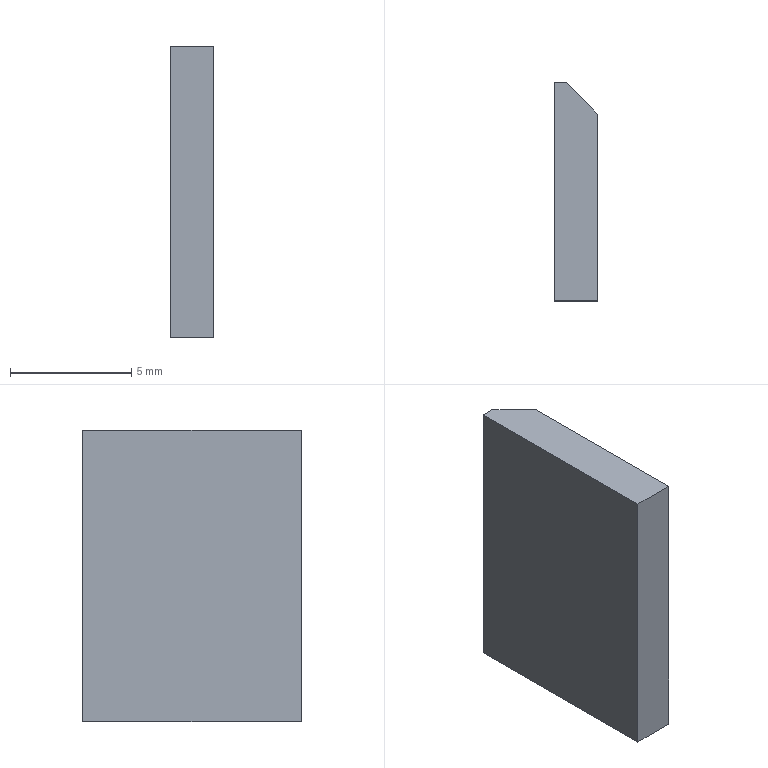Part | SolidWorks | features Extrusion 1 | 1 solid | 7 faces | box 1.8 x 9 x 12 mm | volume 184.26 mm3 | plane 7
STEP:
#1=CARTESIAN_POINT('',(0.5,9.,0.));
#2=VERTEX_POINT('',#1);
#3=CARTESIAN_POINT('',(0.,9.,0.));
#4=VERTEX_POINT('',#3);
#5=CARTESIAN_POINT('',(0.5,9.,0.));
#6=DIRECTION('',(-1.,0.,0.));
#7=VECTOR('',#6,1000.);
#8=LINE('',#5,#7);
#9=EDGE_CURVE('',#2,#4,#8,.T.);
#10=ORIENTED_EDGE('',*,*,#9,.T.);
#11=CARTESIAN_POINT('',(0.,9.,12.));
#12=VERTEX_POINT('',#11);
#13=CARTESIAN_POINT('',(0.,9.,12.));
#14=DIRECTION('',(0.,0.,-1.));
#15=VECTOR('',#14,1000.);
#16=LINE('',#13,#15);
#17=EDGE_CURVE('',#12,#4,#16,.T.);
#18=ORIENTED_EDGE('',*,*,#17,.F.);
#19=CARTESIAN_POINT('',(0.5,9.,12.));
#20=VERTEX_POINT('',#19);
#21=CARTESIAN_POINT('',(0.5,9.,12.));
#22=DIRECTION('',(-1.,0.,0.));
#23=VECTOR('',#22,1000.);
#24=LINE('',#21,#23);
#25=EDGE_CURVE('',#20,#12,#24,.T.);
#26=ORIENTED_EDGE('',*,*,#25,.F.);
#27=CARTESIAN_POINT('',(0.5,9.,12.));
#28=DIRECTION('',(0.,0.,-1.));
#29=VECTOR('',#28,1000.);
#30=LINE('',#27,#29);
#31=EDGE_CURVE('',#20,#2,#30,.T.);
#32=ORIENTED_EDGE('',*,*,#31,.T.);
#33=EDGE_LOOP('',(#10,#18,#26,#32));
#34=FACE_OUTER_BOUND('',#33,.T.);
#35=CARTESIAN_POINT('',(0.5,9.,12.));
#36=DIRECTION('',(0.,-1.,0.));
#37=DIRECTION('',(0.,0.,-1.));
#38=AXIS2_PLACEMENT_3D('',#35,#36,#37);
#39=PLANE('',#38);
#40=ADVANCED_FACE('',(#34),#39,.F.);
#41=CARTESIAN_POINT('',(0.,0.,0.));
#42=VERTEX_POINT('',#41);
#43=CARTESIAN_POINT('',(0.,9.,0.));
#44=DIRECTION('',(0.,-1.,0.));
#45=VECTOR('',#44,1000.);
#46=LINE('',#43,#45);
#47=EDGE_CURVE('',#4,#42,#46,.T.);
#48=ORIENTED_EDGE('',*,*,#47,.T.);
#49=CARTESIAN_POINT('',(0.,0.,12.));
#50=VERTEX_POINT('',#49);
#51=CARTESIAN_POINT('',(0.,0.,12.));
#52=DIRECTION('',(0.,0.,-1.));
#53=VECTOR('',#52,1000.);
#54=LINE('',#51,#53);
#55=EDGE_CURVE('',#50,#42,#54,.T.);
#56=ORIENTED_EDGE('',*,*,#55,.F.);
#57=CARTESIAN_POINT('',(0.,9.,12.));
#58=DIRECTION('',(0.,-1.,0.));
#59=VECTOR('',#58,1000.);
#60=LINE('',#57,#59);
#61=EDGE_CURVE('',#12,#50,#60,.T.);
#62=ORIENTED_EDGE('',*,*,#61,.F.);
#63=ORIENTED_EDGE('',*,*,#17,.T.);
#64=EDGE_LOOP('',(#48,#56,#62,#63));
#65=FACE_OUTER_BOUND('',#64,.T.);
#66=CARTESIAN_POINT('',(0.,9.,12.));
#67=DIRECTION('',(1.,0.,0.));
#68=DIRECTION('',(0.,0.,-1.));
#69=AXIS2_PLACEMENT_3D('',#66,#67,#68);
#70=PLANE('',#69);
#71=ADVANCED_FACE('',(#65),#70,.F.);
#72=CARTESIAN_POINT('',(1.8,0.,0.));
#73=VERTEX_POINT('',#72);
#74=CARTESIAN_POINT('',(0.,0.,0.));
#75=DIRECTION('',(1.,0.,0.));
#76=VECTOR('',#75,1000.);
#77=LINE('',#74,#76);
#78=EDGE_CURVE('',#42,#73,#77,.T.);
#79=ORIENTED_EDGE('',*,*,#78,.T.);
#80=CARTESIAN_POINT('',(1.8,0.,12.));
#81=VERTEX_POINT('',#80);
#82=CARTESIAN_POINT('',(1.8,0.,12.));
#83=DIRECTION('',(0.,0.,-1.));
#84=VECTOR('',#83,1000.);
#85=LINE('',#82,#84);
#86=EDGE_CURVE('',#81,#73,#85,.T.);
#87=ORIENTED_EDGE('',*,*,#86,.F.);
#88=CARTESIAN_POINT('',(0.,0.,12.));
#89=DIRECTION('',(1.,0.,0.));
#90=VECTOR('',#89,1000.);
#91=LINE('',#88,#90);
#92=EDGE_CURVE('',#50,#81,#91,.T.);
#93=ORIENTED_EDGE('',*,*,#92,.F.);
#94=ORIENTED_EDGE('',*,*,#55,.T.);
#95=EDGE_LOOP('',(#79,#87,#93,#94));
#96=FACE_OUTER_BOUND('',#95,.T.);
#97=CARTESIAN_POINT('',(0.,0.,12.));
#98=DIRECTION('',(0.,1.,0.));
#99=DIRECTION('',(0.,0.,1.));
#100=AXIS2_PLACEMENT_3D('',#97,#98,#99);
#101=PLANE('',#100);
#102=ADVANCED_FACE('',(#96),#101,.F.);
#103=CARTESIAN_POINT('',(1.8,7.7,0.));
#104=VERTEX_POINT('',#103);
#105=CARTESIAN_POINT('',(1.8,0.,0.));
#106=DIRECTION('',(0.,1.,0.));
#107=VECTOR('',#106,1000.);
#108=LINE('',#105,#107);
#109=EDGE_CURVE('',#73,#104,#108,.T.);
#110=ORIENTED_EDGE('',*,*,#109,.T.);
#111=CARTESIAN_POINT('',(1.8,7.7,12.));
#112=VERTEX_POINT('',#111);
#113=CARTESIAN_POINT('',(1.8,7.7,12.));
#114=DIRECTION('',(0.,0.,-1.));
#115=VECTOR('',#114,1000.);
#116=LINE('',#113,#115);
#117=EDGE_CURVE('',#112,#104,#116,.T.);
#118=ORIENTED_EDGE('',*,*,#117,.F.);
#119=CARTESIAN_POINT('',(1.8,0.,12.));
#120=DIRECTION('',(0.,1.,0.));
#121=VECTOR('',#120,1000.);
#122=LINE('',#119,#121);
#123=EDGE_CURVE('',#81,#112,#122,.T.);
#124=ORIENTED_EDGE('',*,*,#123,.F.);
#125=ORIENTED_EDGE('',*,*,#86,.T.);
#126=EDGE_LOOP('',(#110,#118,#124,#125));
#127=FACE_OUTER_BOUND('',#126,.T.);
#128=CARTESIAN_POINT('',(1.8,0.,12.));
#129=DIRECTION('',(-1.,0.,0.));
#130=DIRECTION('',(0.,-1.,0.));
#131=AXIS2_PLACEMENT_3D('',#128,#129,#130);
#132=PLANE('',#131);
#133=ADVANCED_FACE('',(#127),#132,.F.);
#134=CARTESIAN_POINT('',(1.8,7.7,0.));
#135=DIRECTION('',(-0.7071,0.7071,0.));
#136=VECTOR('',#135,1000.);
#137=LINE('',#134,#136);
#138=EDGE_CURVE('',#104,#2,#137,.T.);
#139=ORIENTED_EDGE('',*,*,#138,.T.);
#140=ORIENTED_EDGE('',*,*,#31,.F.);
#141=CARTESIAN_POINT('',(1.8,7.7,12.));
#142=DIRECTION('',(-0.7071,0.7071,0.));
#143=VECTOR('',#142,1000.);
#144=LINE('',#141,#143);
#145=EDGE_CURVE('',#112,#20,#144,.T.);
#146=ORIENTED_EDGE('',*,*,#145,.F.);
#147=ORIENTED_EDGE('',*,*,#117,.T.);
#148=EDGE_LOOP('',(#139,#140,#146,#147));
#149=FACE_OUTER_BOUND('',#148,.T.);
#150=CARTESIAN_POINT('',(1.8,7.7,12.));
#151=DIRECTION('',(-0.7071,-0.7071,0.));
#152=DIRECTION('',(0.7071,-0.7071,0.));
#153=AXIS2_PLACEMENT_3D('',#150,#151,#152);
#154=PLANE('',#153);
#155=ADVANCED_FACE('',(#149),#154,.F.);
#156=ORIENTED_EDGE('',*,*,#25,.T.);
#157=ORIENTED_EDGE('',*,*,#61,.T.);
#158=ORIENTED_EDGE('',*,*,#92,.T.);
#159=ORIENTED_EDGE('',*,*,#123,.T.);
#160=ORIENTED_EDGE('',*,*,#145,.T.);
#161=EDGE_LOOP('',(#156,#157,#158,#159,#160));
#162=FACE_OUTER_BOUND('',#161,.T.);
#163=CARTESIAN_POINT('',(0.,0.,12.));
#164=DIRECTION('',(0.,0.,1.));
#165=DIRECTION('',(1.,0.,0.));
#166=AXIS2_PLACEMENT_3D('',#163,#164,#165);
#167=PLANE('',#166);
#168=ADVANCED_FACE('',(#162),#167,.T.);
#169=ORIENTED_EDGE('',*,*,#9,.F.);
#170=ORIENTED_EDGE('',*,*,#138,.F.);
#171=ORIENTED_EDGE('',*,*,#109,.F.);
#172=ORIENTED_EDGE('',*,*,#78,.F.);
#173=ORIENTED_EDGE('',*,*,#47,.F.);
#174=EDGE_LOOP('',(#169,#170,#171,#172,#173));
#175=FACE_OUTER_BOUND('',#174,.T.);
#176=CARTESIAN_POINT('',(0.,0.,0.));
#177=DIRECTION('',(0.,0.,1.));
#178=DIRECTION('',(1.,0.,0.));
#179=AXIS2_PLACEMENT_3D('',#176,#177,#178);
#180=PLANE('',#179);
#181=ADVANCED_FACE('',(#175),#180,.F.);
#182=CLOSED_SHELL('',(#40,#71,#102,#133,#155,#168,#181));
#183=MANIFOLD_SOLID_BREP('',#182);
#184=CARTESIAN_POINT('',(0.,0.,0.));
#185=DIRECTION('',(0.,0.,1.));
#186=DIRECTION('',(1.,0.,0.));
#187=AXIS2_PLACEMENT_3D('',#184,#185,#186);
#188=(LENGTH_UNIT()NAMED_UNIT(*)SI_UNIT(.MILLI.,.METRE.));
#189=UNCERTAINTY_MEASURE_WITH_UNIT(LENGTH_MEASURE(0.00001),#188,'','');
#190=(NAMED_UNIT(*)PLANE_ANGLE_UNIT()SI_UNIT($,.RADIAN.));
#191=(NAMED_UNIT(*)SI_UNIT($,.STERADIAN.)SOLID_ANGLE_UNIT());
#192=(GEOMETRIC_REPRESENTATION_CONTEXT(3)GLOBAL_UNCERTAINTY_ASSIGNED_CONTEXT((#189))GLOBAL_UNIT_ASSIGNED_CONTEXT((#188,#190,#191))REPRESENTATION_CONTEXT('',''));
#193=ADVANCED_BREP_SHAPE_REPRESENTATION('',(#183,#187),#192);